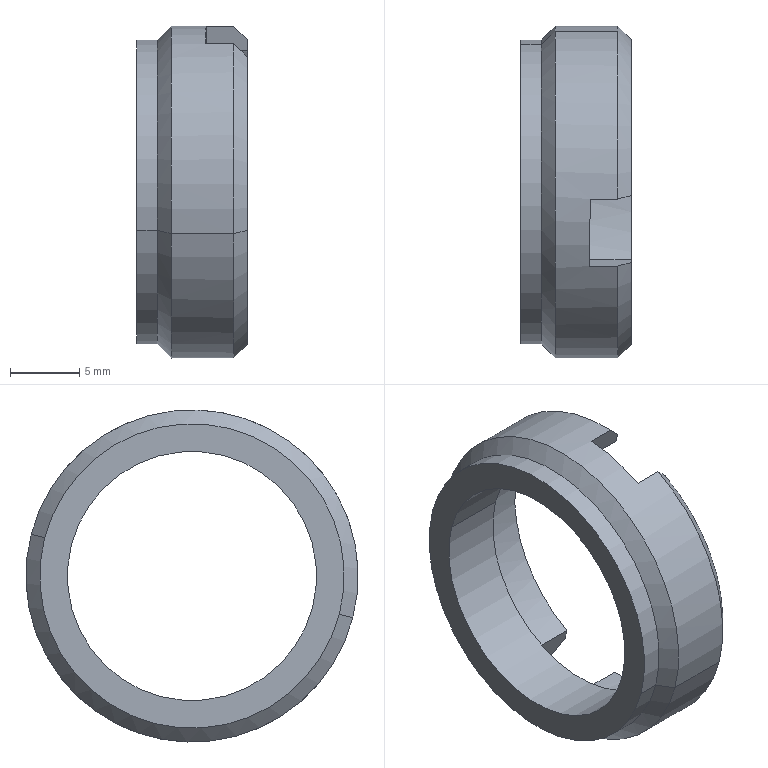Part | SolidWorks | features BaseBody 1 | 1 solid | 23 faces | box 8 x 24 x 24 mm | volume 1089 mm3 | plane 10 | cylinder 8 | cone 5 | commonest cylinder face diameters 18 x2 20.5 x2 22 x2 24 x2
STEP:
#1=CARTESIAN_POINT('',(259.5,87.353,-18.764));
#2=VERTEX_POINT('',#1);
#3=CARTESIAN_POINT('',(259.5,108.647,-13.236));
#4=VERTEX_POINT('',#3);
#5=CARTESIAN_POINT('',(259.5,98.,-16.));
#6=DIRECTION('',(-1.,0.,0.));
#7=DIRECTION('',(0.,-0.9679,-0.2513));
#8=AXIS2_PLACEMENT_3D('',#5,#6,#7);
#9=CIRCLE('',#8,11.);
#10=EDGE_CURVE('',#2,#4,#9,.T.);
#11=ORIENTED_EDGE('',*,*,#10,.F.);
#12=CARTESIAN_POINT('',(260.5,86.385,-19.015));
#13=VERTEX_POINT('',#12);
#14=CARTESIAN_POINT('',(259.5,87.353,-18.764));
#15=DIRECTION('',(0.7071,-0.6844,-0.1777));
#16=VECTOR('',#15,1000.);
#17=LINE('',#14,#16);
#18=EDGE_CURVE('',#2,#13,#17,.T.);
#19=ORIENTED_EDGE('',*,*,#18,.T.);
#20=CARTESIAN_POINT('',(260.5,109.615,-12.985));
#21=VERTEX_POINT('',#20);
#22=CARTESIAN_POINT('',(260.5,98.,-16.));
#23=DIRECTION('',(1.,0.,0.));
#24=DIRECTION('',(0.,-0.9679,-0.2513));
#25=AXIS2_PLACEMENT_3D('',#22,#23,#24);
#26=CIRCLE('',#25,12.);
#27=EDGE_CURVE('',#21,#13,#26,.T.);
#28=ORIENTED_EDGE('',*,*,#27,.F.);
#29=CARTESIAN_POINT('',(259.5,108.647,-13.236));
#30=DIRECTION('',(0.7071,0.6844,0.1777));
#31=VECTOR('',#30,1000.);
#32=LINE('',#29,#31);
#33=EDGE_CURVE('',#4,#21,#32,.T.);
#34=ORIENTED_EDGE('',*,*,#33,.F.);
#35=EDGE_LOOP('',(#11,#19,#28,#34));
#36=FACE_OUTER_BOUND('',#35,.T.);
#37=CARTESIAN_POINT('',(259.5,98.,-16.));
#38=DIRECTION('',(1.,0.,0.));
#39=DIRECTION('',(0.,0.9679,0.2513));
#40=AXIS2_PLACEMENT_3D('',#37,#38,#39);
#41=CONICAL_SURFACE('',#40,11.,0.7854);
#42=ADVANCED_FACE('',(#36),#41,.T.);
#43=CARTESIAN_POINT('',(266.,87.353,-18.764));
#44=VERTEX_POINT('',#43);
#45=CARTESIAN_POINT('',(266.,98.272,-26.997));
#46=VERTEX_POINT('',#45);
#47=CARTESIAN_POINT('',(266.,98.,-16.));
#48=DIRECTION('',(1.,0.,0.));
#49=DIRECTION('',(0.,-0.9679,-0.2513));
#50=AXIS2_PLACEMENT_3D('',#47,#48,#49);
#51=CIRCLE('',#50,11.);
#52=EDGE_CURVE('',#44,#46,#51,.T.);
#53=ORIENTED_EDGE('',*,*,#52,.F.);
#54=CARTESIAN_POINT('',(265.,86.385,-19.015));
#55=VERTEX_POINT('',#54);
#56=CARTESIAN_POINT('',(265.,86.385,-19.015));
#57=DIRECTION('',(-0.7071,-0.6844,-0.1777));
#58=VECTOR('',#57,1000.);
#59=LINE('',#56,#58);
#60=EDGE_CURVE('',#44,#55,#59,.T.);
#61=ORIENTED_EDGE('',*,*,#60,.T.);
#62=CARTESIAN_POINT('',(265.,98.529,-27.988));
#63=VERTEX_POINT('',#62);
#64=CARTESIAN_POINT('',(265.,98.,-16.));
#65=DIRECTION('',(-1.,0.,0.));
#66=DIRECTION('',(0.,-0.9679,-0.2513));
#67=AXIS2_PLACEMENT_3D('',#64,#65,#66);
#68=CIRCLE('',#67,12.);
#69=EDGE_CURVE('',#63,#55,#68,.T.);
#70=ORIENTED_EDGE('',*,*,#69,.F.);
#71=CARTESIAN_POINT('',(266.,98.272,-26.997));
#72=CARTESIAN_POINT('',(265.667,98.358,-27.328));
#73=CARTESIAN_POINT('',(265.334,98.443,-27.658));
#74=CARTESIAN_POINT('',(265.,98.529,-27.988));
#75=B_SPLINE_CURVE_WITH_KNOTS('',3,(#71,#72,#73,#74),.UNSPECIFIED.,.F.,.F.,(4,4),(0.04958,0.051),.UNSPECIFIED.);
#76=EDGE_CURVE('',#46,#63,#75,.T.);
#77=ORIENTED_EDGE('',*,*,#76,.F.);
#78=EDGE_LOOP('',(#53,#61,#70,#77));
#79=FACE_OUTER_BOUND('',#78,.T.);
#80=CARTESIAN_POINT('',(265.,98.,-16.));
#81=DIRECTION('',(-1.,0.,0.));
#82=DIRECTION('',(0.,-0.9679,-0.2513));
#83=AXIS2_PLACEMENT_3D('',#80,#81,#82);
#84=CONICAL_SURFACE('',#83,12.,0.7854);
#85=ADVANCED_FACE('',(#79),#84,.T.);
#86=CARTESIAN_POINT('',(258.,89.289,-18.261));
#87=VERTEX_POINT('',#86);
#88=CARTESIAN_POINT('',(258.,106.711,-13.739));
#89=VERTEX_POINT('',#88);
#90=CARTESIAN_POINT('',(258.,98.,-16.));
#91=DIRECTION('',(1.,0.,0.));
#92=DIRECTION('',(0.,0.9679,0.2513));
#93=AXIS2_PLACEMENT_3D('',#90,#91,#92);
#94=CIRCLE('',#93,9.);
#95=EDGE_CURVE('',#87,#89,#94,.T.);
#96=ORIENTED_EDGE('',*,*,#95,.F.);
#97=CARTESIAN_POINT('',(262.5,89.289,-18.261));
#98=VERTEX_POINT('',#97);
#99=CARTESIAN_POINT('',(258.,89.289,-18.261));
#100=DIRECTION('',(1.,0.,0.));
#101=VECTOR('',#100,1000.);
#102=LINE('',#99,#101);
#103=EDGE_CURVE('',#87,#98,#102,.T.);
#104=ORIENTED_EDGE('',*,*,#103,.T.);
#105=CARTESIAN_POINT('',(262.5,106.711,-13.739));
#106=VERTEX_POINT('',#105);
#107=CARTESIAN_POINT('',(262.5,98.,-16.));
#108=DIRECTION('',(1.,0.,0.));
#109=DIRECTION('',(0.,0.9679,0.2513));
#110=AXIS2_PLACEMENT_3D('',#107,#108,#109);
#111=CIRCLE('',#110,9.);
#112=EDGE_CURVE('',#98,#106,#111,.T.);
#113=ORIENTED_EDGE('',*,*,#112,.T.);
#114=CARTESIAN_POINT('',(258.,106.711,-13.739));
#115=DIRECTION('',(1.,0.,0.));
#116=VECTOR('',#115,1000.);
#117=LINE('',#114,#116);
#118=EDGE_CURVE('',#89,#106,#117,.T.);
#119=ORIENTED_EDGE('',*,*,#118,.F.);
#120=EDGE_LOOP('',(#96,#104,#113,#119));
#121=FACE_OUTER_BOUND('',#120,.T.);
#122=CARTESIAN_POINT('',(258.,98.,-16.));
#123=DIRECTION('',(1.,0.,0.));
#124=DIRECTION('',(0.,0.9679,0.2513));
#125=AXIS2_PLACEMENT_3D('',#122,#123,#124);
#126=CYLINDRICAL_SURFACE('',#125,9.);
#127=ADVANCED_FACE('',(#121),#126,.F.);
#128=CARTESIAN_POINT('',(262.5,88.079,-18.575));
#129=VERTEX_POINT('',#128);
#130=CARTESIAN_POINT('',(262.5,107.921,-13.425));
#131=VERTEX_POINT('',#130);
#132=CARTESIAN_POINT('',(262.5,98.,-16.));
#133=DIRECTION('',(1.,0.,0.));
#134=DIRECTION('',(0.,0.9679,0.2513));
#135=AXIS2_PLACEMENT_3D('',#132,#133,#134);
#136=CIRCLE('',#135,10.25);
#137=EDGE_CURVE('',#129,#131,#136,.T.);
#138=ORIENTED_EDGE('',*,*,#137,.F.);
#139=CARTESIAN_POINT('',(266.,88.079,-18.575));
#140=VERTEX_POINT('',#139);
#141=CARTESIAN_POINT('',(262.5,88.079,-18.575));
#142=DIRECTION('',(1.,0.,0.));
#143=VECTOR('',#142,1000.);
#144=LINE('',#141,#143);
#145=EDGE_CURVE('',#129,#140,#144,.T.);
#146=ORIENTED_EDGE('',*,*,#145,.T.);
#147=CARTESIAN_POINT('',(266.,98.078,-26.25));
#148=VERTEX_POINT('',#147);
#149=CARTESIAN_POINT('',(266.,98.,-16.));
#150=DIRECTION('',(1.,0.,0.));
#151=DIRECTION('',(0.,0.9679,0.2513));
#152=AXIS2_PLACEMENT_3D('',#149,#150,#151);
#153=CIRCLE('',#152,10.25);
#154=EDGE_CURVE('',#140,#148,#153,.T.);
#155=ORIENTED_EDGE('',*,*,#154,.T.);
#156=CARTESIAN_POINT('',(262.973,98.078,-26.25));
#157=VERTEX_POINT('',#156);
#158=CARTESIAN_POINT('',(262.5,98.078,-26.25));
#159=DIRECTION('',(-1.,0.,0.));
#160=VECTOR('',#159,1000.);
#161=LINE('',#158,#160);
#162=EDGE_CURVE('',#148,#157,#161,.T.);
#163=ORIENTED_EDGE('',*,*,#162,.T.);
#164=CARTESIAN_POINT('',(263.027,102.917,-24.993));
#165=VERTEX_POINT('',#164);
#166=CARTESIAN_POINT('',(262.973,98.078,-26.25));
#167=CARTESIAN_POINT('',(262.991,99.779,-26.237));
#168=CARTESIAN_POINT('',(263.009,101.425,-25.809));
#169=CARTESIAN_POINT('',(263.027,102.917,-24.993));
#170=(BOUNDED_CURVE()B_SPLINE_CURVE(3,(#166,#167,#168,#169),.UNSPECIFIED.,.F.,.F.)B_SPLINE_CURVE_WITH_KNOTS((4,4),(4.466,4.959),.UNSPECIFIED.)CURVE()GEOMETRIC_REPRESENTATION_ITEM()RATIONAL_B_SPLINE_CURVE((1.,0.9799,0.9799,1.))REPRESENTATION_ITEM(''));
#171=EDGE_CURVE('',#157,#165,#170,.T.);
#172=ORIENTED_EDGE('',*,*,#171,.T.);
#173=CARTESIAN_POINT('',(266.,102.917,-24.993));
#174=VERTEX_POINT('',#173);
#175=CARTESIAN_POINT('',(262.5,102.917,-24.993));
#176=DIRECTION('',(1.,0.,0.));
#177=VECTOR('',#176,1000.);
#178=LINE('',#175,#177);
#179=EDGE_CURVE('',#165,#174,#178,.T.);
#180=ORIENTED_EDGE('',*,*,#179,.T.);
#181=CARTESIAN_POINT('',(266.,107.921,-13.425));
#182=VERTEX_POINT('',#181);
#183=CARTESIAN_POINT('',(266.,98.,-16.));
#184=DIRECTION('',(1.,0.,0.));
#185=DIRECTION('',(0.,0.9679,0.2513));
#186=AXIS2_PLACEMENT_3D('',#183,#184,#185);
#187=CIRCLE('',#186,10.25);
#188=EDGE_CURVE('',#174,#182,#187,.T.);
#189=ORIENTED_EDGE('',*,*,#188,.T.);
#190=CARTESIAN_POINT('',(262.5,107.921,-13.425));
#191=DIRECTION('',(1.,0.,0.));
#192=VECTOR('',#191,1000.);
#193=LINE('',#190,#192);
#194=EDGE_CURVE('',#131,#182,#193,.T.);
#195=ORIENTED_EDGE('',*,*,#194,.F.);
#196=EDGE_LOOP('',(#138,#146,#155,#163,#172,#180,#189,#195));
#197=FACE_OUTER_BOUND('',#196,.T.);
#198=CARTESIAN_POINT('',(262.5,98.,-16.));
#199=DIRECTION('',(1.,0.,0.));
#200=DIRECTION('',(0.,0.9679,0.2513));
#201=AXIS2_PLACEMENT_3D('',#198,#199,#200);
#202=CYLINDRICAL_SURFACE('',#201,10.25);
#203=ADVANCED_FACE('',(#197),#202,.F.);
#204=CARTESIAN_POINT('',(258.,87.353,-18.764));
#205=VERTEX_POINT('',#204);
#206=CARTESIAN_POINT('',(258.,108.647,-13.236));
#207=VERTEX_POINT('',#206);
#208=CARTESIAN_POINT('',(258.,98.,-16.));
#209=DIRECTION('',(-1.,0.,0.));
#210=DIRECTION('',(0.,-0.9679,-0.2513));
#211=AXIS2_PLACEMENT_3D('',#208,#209,#210);
#212=CIRCLE('',#211,11.);
#213=EDGE_CURVE('',#205,#207,#212,.T.);
#214=ORIENTED_EDGE('',*,*,#213,.F.);
#215=CARTESIAN_POINT('',(258.,87.353,-18.764));
#216=DIRECTION('',(1.,0.,0.));
#217=VECTOR('',#216,1000.);
#218=LINE('',#215,#217);
#219=EDGE_CURVE('',#205,#2,#218,.T.);
#220=ORIENTED_EDGE('',*,*,#219,.T.);
#221=ORIENTED_EDGE('',*,*,#10,.T.);
#222=CARTESIAN_POINT('',(258.,108.647,-13.236));
#223=DIRECTION('',(1.,0.,0.));
#224=VECTOR('',#223,1000.);
#225=LINE('',#222,#224);
#226=EDGE_CURVE('',#207,#4,#225,.T.);
#227=ORIENTED_EDGE('',*,*,#226,.F.);
#228=EDGE_LOOP('',(#214,#220,#221,#227));
#229=FACE_OUTER_BOUND('',#228,.T.);
#230=CARTESIAN_POINT('',(258.,98.,-16.));
#231=DIRECTION('',(1.,0.,0.));
#232=DIRECTION('',(0.,0.9679,0.2513));
#233=AXIS2_PLACEMENT_3D('',#230,#231,#232);
#234=CYLINDRICAL_SURFACE('',#233,11.);
#235=ADVANCED_FACE('',(#229),#234,.T.);
#236=ORIENTED_EDGE('',*,*,#27,.T.);
#237=CARTESIAN_POINT('',(259.5,86.385,-19.015));
#238=DIRECTION('',(1.,0.,0.));
#239=VECTOR('',#238,1000.);
#240=LINE('',#237,#239);
#241=EDGE_CURVE('',#13,#55,#240,.T.);
#242=ORIENTED_EDGE('',*,*,#241,.T.);
#243=CARTESIAN_POINT('',(265.,92.631,-5.268));
#244=VERTEX_POINT('',#243);
#245=CARTESIAN_POINT('',(265.,98.,-16.));
#246=DIRECTION('',(-1.,0.,0.));
#247=DIRECTION('',(0.,-0.9679,-0.2513));
#248=AXIS2_PLACEMENT_3D('',#245,#246,#247);
#249=CIRCLE('',#248,12.);
#250=EDGE_CURVE('',#55,#244,#249,.T.);
#251=ORIENTED_EDGE('',*,*,#250,.T.);
#252=CARTESIAN_POINT('',(262.973,92.631,-5.268));
#253=VERTEX_POINT('',#252);
#254=CARTESIAN_POINT('',(259.5,92.631,-5.268));
#255=DIRECTION('',(-1.,0.,0.));
#256=VECTOR('',#255,1000.);
#257=LINE('',#254,#256);
#258=EDGE_CURVE('',#244,#253,#257,.T.);
#259=ORIENTED_EDGE('',*,*,#258,.T.);
#260=CARTESIAN_POINT('',(263.027,97.471,-4.012));
#261=VERTEX_POINT('',#260);
#262=CARTESIAN_POINT('',(262.973,92.631,-5.268));
#263=CARTESIAN_POINT('',(262.991,94.144,-4.511));
#264=CARTESIAN_POINT('',(263.009,95.781,-4.086));
#265=CARTESIAN_POINT('',(263.027,97.471,-4.012));
#266=(BOUNDED_CURVE()B_SPLINE_CURVE(3,(#262,#263,#264,#265),.UNSPECIFIED.,.F.,.T.)B_SPLINE_CURVE_WITH_KNOTS((4,4),(4.503,4.922),.UNSPECIFIED.)CURVE()GEOMETRIC_REPRESENTATION_ITEM()RATIONAL_B_SPLINE_CURVE((1.,0.9854,0.9854,1.))REPRESENTATION_ITEM(''));
#267=EDGE_CURVE('',#253,#261,#266,.T.);
#268=ORIENTED_EDGE('',*,*,#267,.T.);
#269=CARTESIAN_POINT('',(265.,97.471,-4.012));
#270=VERTEX_POINT('',#269);
#271=CARTESIAN_POINT('',(259.5,97.471,-4.012));
#272=DIRECTION('',(1.,0.,0.));
#273=VECTOR('',#272,1000.);
#274=LINE('',#271,#273);
#275=EDGE_CURVE('',#261,#270,#274,.T.);
#276=ORIENTED_EDGE('',*,*,#275,.T.);
#277=CARTESIAN_POINT('',(265.,109.615,-12.985));
#278=VERTEX_POINT('',#277);
#279=CARTESIAN_POINT('',(265.,98.,-16.));
#280=DIRECTION('',(-1.,0.,0.));
#281=DIRECTION('',(0.,-0.9679,-0.2513));
#282=AXIS2_PLACEMENT_3D('',#279,#280,#281);
#283=CIRCLE('',#282,12.);
#284=EDGE_CURVE('',#270,#278,#283,.T.);
#285=ORIENTED_EDGE('',*,*,#284,.T.);
#286=CARTESIAN_POINT('',(259.5,109.615,-12.985));
#287=DIRECTION('',(1.,0.,0.));
#288=VECTOR('',#287,1000.);
#289=LINE('',#286,#288);
#290=EDGE_CURVE('',#21,#278,#289,.T.);
#291=ORIENTED_EDGE('',*,*,#290,.F.);
#292=EDGE_LOOP('',(#236,#242,#251,#259,#268,#276,#285,#291));
#293=FACE_OUTER_BOUND('',#292,.T.);
#294=CARTESIAN_POINT('',(259.5,98.,-16.));
#295=DIRECTION('',(1.,0.,0.));
#296=DIRECTION('',(0.,0.9679,0.2513));
#297=AXIS2_PLACEMENT_3D('',#294,#295,#296);
#298=CYLINDRICAL_SURFACE('',#297,12.);
#299=ADVANCED_FACE('',(#293),#298,.T.);
#300=CARTESIAN_POINT('',(266.,103.111,-25.74));
#301=VERTEX_POINT('',#300);
#302=CARTESIAN_POINT('',(266.,97.728,-5.003));
#303=VERTEX_POINT('',#302);
#304=CARTESIAN_POINT('',(266.,98.,-16.));
#305=DIRECTION('',(1.,0.,0.));
#306=DIRECTION('',(0.,-0.9679,-0.2513));
#307=AXIS2_PLACEMENT_3D('',#304,#305,#306);
#308=CIRCLE('',#307,11.);
#309=EDGE_CURVE('',#301,#303,#308,.T.);
#310=ORIENTED_EDGE('',*,*,#309,.T.);
#311=CARTESIAN_POINT('',(266.,97.922,-5.75));
#312=VERTEX_POINT('',#311);
#313=CARTESIAN_POINT('',(266.,103.435,-26.987));
#314=DIRECTION('',(0.,-0.2513,0.9679));
#315=VECTOR('',#314,1000.);
#316=LINE('',#313,#315);
#317=EDGE_CURVE('',#312,#303,#316,.T.);
#318=ORIENTED_EDGE('',*,*,#317,.F.);
#319=CARTESIAN_POINT('',(266.,98.,-16.));
#320=DIRECTION('',(1.,0.,0.));
#321=DIRECTION('',(0.,0.9679,0.2513));
#322=AXIS2_PLACEMENT_3D('',#319,#320,#321);
#323=CIRCLE('',#322,10.25);
#324=EDGE_CURVE('',#182,#312,#323,.T.);
#325=ORIENTED_EDGE('',*,*,#324,.F.);
#326=ORIENTED_EDGE('',*,*,#188,.F.);
#327=CARTESIAN_POINT('',(266.,103.435,-26.987));
#328=DIRECTION('',(0.,-0.2513,0.9679));
#329=VECTOR('',#328,1000.);
#330=LINE('',#327,#329);
#331=EDGE_CURVE('',#301,#174,#330,.T.);
#332=ORIENTED_EDGE('',*,*,#331,.F.);
#333=EDGE_LOOP('',(#310,#318,#325,#326,#332));
#334=FACE_OUTER_BOUND('',#333,.T.);
#335=CARTESIAN_POINT('',(266.,98.,-16.));
#336=DIRECTION('',(-1.,0.,0.));
#337=DIRECTION('',(0.,-0.9679,-0.2513));
#338=AXIS2_PLACEMENT_3D('',#335,#336,#337);
#339=PLANE('',#338);
#340=ADVANCED_FACE('',(#334),#339,.F.);
#341=CARTESIAN_POINT('',(265.,103.369,-26.732));
#342=VERTEX_POINT('',#341);
#343=CARTESIAN_POINT('',(265.,103.369,-26.732));
#344=CARTESIAN_POINT('',(265.334,103.283,-26.402));
#345=CARTESIAN_POINT('',(265.667,103.197,-26.071));
#346=CARTESIAN_POINT('',(266.,103.111,-25.74));
#347=B_SPLINE_CURVE_WITH_KNOTS('',3,(#343,#344,#345,#346),.UNSPECIFIED.,.F.,.F.,(4,4),(0.02048,0.02192),.UNSPECIFIED.);
#348=EDGE_CURVE('',#342,#301,#347,.T.);
#349=ORIENTED_EDGE('',*,*,#348,.F.);
#350=CARTESIAN_POINT('',(265.,98.,-16.));
#351=DIRECTION('',(-1.,0.,0.));
#352=DIRECTION('',(0.,-0.9679,-0.2513));
#353=AXIS2_PLACEMENT_3D('',#350,#351,#352);
#354=CIRCLE('',#353,12.);
#355=EDGE_CURVE('',#278,#342,#354,.T.);
#356=ORIENTED_EDGE('',*,*,#355,.F.);
#357=ORIENTED_EDGE('',*,*,#284,.F.);
#358=CARTESIAN_POINT('',(266.,97.728,-5.003));
#359=CARTESIAN_POINT('',(265.667,97.642,-4.672));
#360=CARTESIAN_POINT('',(265.334,97.557,-4.342));
#361=CARTESIAN_POINT('',(265.,97.471,-4.012));
#362=B_SPLINE_CURVE_WITH_KNOTS('',3,(#358,#359,#360,#361),.UNSPECIFIED.,.F.,.F.,(4,4),(0.04958,0.051),.UNSPECIFIED.);
#363=EDGE_CURVE('',#303,#270,#362,.T.);
#364=ORIENTED_EDGE('',*,*,#363,.F.);
#365=ORIENTED_EDGE('',*,*,#309,.F.);
#366=EDGE_LOOP('',(#349,#356,#357,#364,#365));
#367=FACE_OUTER_BOUND('',#366,.T.);
#368=CARTESIAN_POINT('',(265.,98.,-16.));
#369=DIRECTION('',(-1.,0.,0.));
#370=DIRECTION('',(0.,-0.9679,-0.2513));
#371=AXIS2_PLACEMENT_3D('',#368,#369,#370);
#372=CONICAL_SURFACE('',#371,12.,0.7854);
#373=ADVANCED_FACE('',(#367),#372,.T.);
#374=ORIENTED_EDGE('',*,*,#241,.F.);
#375=CARTESIAN_POINT('',(260.5,98.,-16.));
#376=DIRECTION('',(1.,0.,0.));
#377=DIRECTION('',(0.,-0.9679,-0.2513));
#378=AXIS2_PLACEMENT_3D('',#375,#376,#377);
#379=CIRCLE('',#378,12.);
#380=EDGE_CURVE('',#13,#21,#379,.T.);
#381=ORIENTED_EDGE('',*,*,#380,.T.);
#382=ORIENTED_EDGE('',*,*,#290,.T.);
#383=ORIENTED_EDGE('',*,*,#355,.T.);
#384=CARTESIAN_POINT('',(263.027,103.369,-26.732));
#385=VERTEX_POINT('',#384);
#386=CARTESIAN_POINT('',(259.5,103.369,-26.732));
#387=DIRECTION('',(-1.,0.,0.));
#388=VECTOR('',#387,1000.);
#389=LINE('',#386,#388);
#390=EDGE_CURVE('',#342,#385,#389,.T.);
#391=ORIENTED_EDGE('',*,*,#390,.T.);
#392=CARTESIAN_POINT('',(262.973,98.529,-27.988));
#393=VERTEX_POINT('',#392);
#394=CARTESIAN_POINT('',(263.027,103.369,-26.732));
#395=CARTESIAN_POINT('',(263.009,101.856,-27.489));
#396=CARTESIAN_POINT('',(262.991,100.219,-27.914));
#397=CARTESIAN_POINT('',(262.973,98.529,-27.988));
#398=(BOUNDED_CURVE()B_SPLINE_CURVE(3,(#394,#395,#396,#397),.UNSPECIFIED.,.F.,.F.)B_SPLINE_CURVE_WITH_KNOTS((4,4),(1.361,1.781),.UNSPECIFIED.)CURVE()GEOMETRIC_REPRESENTATION_ITEM()RATIONAL_B_SPLINE_CURVE((1.,0.9854,0.9854,1.))REPRESENTATION_ITEM(''));
#399=EDGE_CURVE('',#385,#393,#398,.T.);
#400=ORIENTED_EDGE('',*,*,#399,.T.);
#401=CARTESIAN_POINT('',(259.5,98.529,-27.988));
#402=DIRECTION('',(1.,0.,0.));
#403=VECTOR('',#402,1000.);
#404=LINE('',#401,#403);
#405=EDGE_CURVE('',#393,#63,#404,.T.);
#406=ORIENTED_EDGE('',*,*,#405,.T.);
#407=ORIENTED_EDGE('',*,*,#69,.T.);
#408=EDGE_LOOP('',(#374,#381,#382,#383,#391,#400,#406,#407));
#409=FACE_OUTER_BOUND('',#408,.T.);
#410=CARTESIAN_POINT('',(259.5,98.,-16.));
#411=DIRECTION('',(1.,0.,0.));
#412=DIRECTION('',(0.,0.9679,0.2513));
#413=AXIS2_PLACEMENT_3D('',#410,#411,#412);
#414=CYLINDRICAL_SURFACE('',#413,12.);
#415=ADVANCED_FACE('',(#409),#414,.T.);
#416=CARTESIAN_POINT('',(266.,92.889,-6.26));
#417=VERTEX_POINT('',#416);
#418=CARTESIAN_POINT('',(266.,98.,-16.));
#419=DIRECTION('',(1.,0.,0.));
#420=DIRECTION('',(0.,-0.9679,-0.2513));
#421=AXIS2_PLACEMENT_3D('',#418,#419,#420);
#422=CIRCLE('',#421,11.);
#423=EDGE_CURVE('',#417,#44,#422,.T.);
#424=ORIENTED_EDGE('',*,*,#423,.T.);
#425=ORIENTED_EDGE('',*,*,#52,.T.);
#426=CARTESIAN_POINT('',(266.,98.595,-28.243));
#427=DIRECTION('',(0.,-0.2513,0.9679));
#428=VECTOR('',#427,1000.);
#429=LINE('',#426,#428);
#430=EDGE_CURVE('',#46,#148,#429,.T.);
#431=ORIENTED_EDGE('',*,*,#430,.T.);
#432=ORIENTED_EDGE('',*,*,#154,.F.);
#433=CARTESIAN_POINT('',(266.,93.083,-7.007));
#434=VERTEX_POINT('',#433);
#435=CARTESIAN_POINT('',(266.,98.,-16.));
#436=DIRECTION('',(1.,0.,0.));
#437=DIRECTION('',(0.,0.9679,0.2513));
#438=AXIS2_PLACEMENT_3D('',#435,#436,#437);
#439=CIRCLE('',#438,10.25);
#440=EDGE_CURVE('',#434,#140,#439,.T.);
#441=ORIENTED_EDGE('',*,*,#440,.F.);
#442=CARTESIAN_POINT('',(266.,98.595,-28.243));
#443=DIRECTION('',(0.,-0.2513,0.9679));
#444=VECTOR('',#443,1000.);
#445=LINE('',#442,#444);
#446=EDGE_CURVE('',#434,#417,#445,.T.);
#447=ORIENTED_EDGE('',*,*,#446,.T.);
#448=EDGE_LOOP('',(#424,#425,#431,#432,#441,#447));
#449=FACE_OUTER_BOUND('',#448,.T.);
#450=CARTESIAN_POINT('',(266.,98.,-16.));
#451=DIRECTION('',(-1.,0.,0.));
#452=DIRECTION('',(0.,-0.9679,-0.2513));
#453=AXIS2_PLACEMENT_3D('',#450,#451,#452);
#454=PLANE('',#453);
#455=ADVANCED_FACE('',(#449),#454,.F.);
#456=ORIENTED_EDGE('',*,*,#219,.F.);
#457=CARTESIAN_POINT('',(258.,98.,-16.));
#458=DIRECTION('',(-1.,0.,0.));
#459=DIRECTION('',(0.,-0.9679,-0.2513));
#460=AXIS2_PLACEMENT_3D('',#457,#458,#459);
#461=CIRCLE('',#460,11.);
#462=EDGE_CURVE('',#207,#205,#461,.T.);
#463=ORIENTED_EDGE('',*,*,#462,.F.);
#464=ORIENTED_EDGE('',*,*,#226,.T.);
#465=CARTESIAN_POINT('',(259.5,98.,-16.));
#466=DIRECTION('',(-1.,0.,0.));
#467=DIRECTION('',(0.,-0.9679,-0.2513));
#468=AXIS2_PLACEMENT_3D('',#465,#466,#467);
#469=CIRCLE('',#468,11.);
#470=EDGE_CURVE('',#4,#2,#469,.T.);
#471=ORIENTED_EDGE('',*,*,#470,.T.);
#472=EDGE_LOOP('',(#456,#463,#464,#471));
#473=FACE_OUTER_BOUND('',#472,.T.);
#474=CARTESIAN_POINT('',(258.,98.,-16.));
#475=DIRECTION('',(1.,0.,0.));
#476=DIRECTION('',(0.,0.9679,0.2513));
#477=AXIS2_PLACEMENT_3D('',#474,#475,#476);
#478=CYLINDRICAL_SURFACE('',#477,11.);
#479=ADVANCED_FACE('',(#473),#478,.T.);
#480=CARTESIAN_POINT('',(258.,98.,-16.));
#481=DIRECTION('',(1.,0.,0.));
#482=DIRECTION('',(0.,0.9679,0.2513));
#483=AXIS2_PLACEMENT_3D('',#480,#481,#482);
#484=CIRCLE('',#483,9.);
#485=EDGE_CURVE('',#89,#87,#484,.T.);
#486=ORIENTED_EDGE('',*,*,#485,.T.);
#487=ORIENTED_EDGE('',*,*,#95,.T.);
#488=EDGE_LOOP('',(#486,#487));
#489=FACE_BOUND('',#488,.T.);
#490=ORIENTED_EDGE('',*,*,#462,.T.);
#491=ORIENTED_EDGE('',*,*,#213,.T.);
#492=EDGE_LOOP('',(#490,#491));
#493=FACE_OUTER_BOUND('',#492,.T.);
#494=CARTESIAN_POINT('',(258.,98.,-16.));
#495=DIRECTION('',(-1.,0.,0.));
#496=DIRECTION('',(0.,-0.9679,-0.2513));
#497=AXIS2_PLACEMENT_3D('',#494,#495,#496);
#498=PLANE('',#497);
#499=ADVANCED_FACE('',(#489,#493),#498,.T.);
#500=ORIENTED_EDGE('',*,*,#145,.F.);
#501=CARTESIAN_POINT('',(262.5,98.,-16.));
#502=DIRECTION('',(1.,0.,0.));
#503=DIRECTION('',(0.,0.9679,0.2513));
#504=AXIS2_PLACEMENT_3D('',#501,#502,#503);
#505=CIRCLE('',#504,10.25);
#506=EDGE_CURVE('',#131,#129,#505,.T.);
#507=ORIENTED_EDGE('',*,*,#506,.F.);
#508=ORIENTED_EDGE('',*,*,#194,.T.);
#509=ORIENTED_EDGE('',*,*,#324,.T.);
#510=CARTESIAN_POINT('',(263.027,97.922,-5.75));
#511=VERTEX_POINT('',#510);
#512=CARTESIAN_POINT('',(262.5,97.922,-5.75));
#513=DIRECTION('',(-1.,0.,0.));
#514=VECTOR('',#513,1000.);
#515=LINE('',#512,#514);
#516=EDGE_CURVE('',#312,#511,#515,.T.);
#517=ORIENTED_EDGE('',*,*,#516,.T.);
#518=CARTESIAN_POINT('',(262.973,93.083,-7.007));
#519=VERTEX_POINT('',#518);
#520=CARTESIAN_POINT('',(263.027,97.922,-5.75));
#521=CARTESIAN_POINT('',(263.009,96.221,-5.763));
#522=CARTESIAN_POINT('',(262.991,94.575,-6.191));
#523=CARTESIAN_POINT('',(262.973,93.083,-7.007));
#524=(BOUNDED_CURVE()B_SPLINE_CURVE(3,(#520,#521,#522,#523),.UNSPECIFIED.,.F.,.F.)B_SPLINE_CURVE_WITH_KNOTS((4,4),(1.324,1.817),.UNSPECIFIED.)CURVE()GEOMETRIC_REPRESENTATION_ITEM()RATIONAL_B_SPLINE_CURVE((1.,0.9799,0.9799,1.))REPRESENTATION_ITEM(''));
#525=EDGE_CURVE('',#511,#519,#524,.T.);
#526=ORIENTED_EDGE('',*,*,#525,.T.);
#527=CARTESIAN_POINT('',(262.5,93.083,-7.007));
#528=DIRECTION('',(1.,0.,0.));
#529=VECTOR('',#528,1000.);
#530=LINE('',#527,#529);
#531=EDGE_CURVE('',#519,#434,#530,.T.);
#532=ORIENTED_EDGE('',*,*,#531,.T.);
#533=ORIENTED_EDGE('',*,*,#440,.T.);
#534=EDGE_LOOP('',(#500,#507,#508,#509,#517,#526,#532,#533));
#535=FACE_OUTER_BOUND('',#534,.T.);
#536=CARTESIAN_POINT('',(262.5,98.,-16.));
#537=DIRECTION('',(1.,0.,0.));
#538=DIRECTION('',(0.,0.9679,0.2513));
#539=AXIS2_PLACEMENT_3D('',#536,#537,#538);
#540=CYLINDRICAL_SURFACE('',#539,10.25);
#541=ADVANCED_FACE('',(#535),#540,.F.);
#542=CARTESIAN_POINT('',(262.5,98.,-16.));
#543=DIRECTION('',(1.,0.,0.));
#544=DIRECTION('',(0.,0.9679,0.2513));
#545=AXIS2_PLACEMENT_3D('',#542,#543,#544);
#546=CIRCLE('',#545,9.);
#547=EDGE_CURVE('',#106,#98,#546,.T.);
#548=ORIENTED_EDGE('',*,*,#547,.F.);
#549=ORIENTED_EDGE('',*,*,#112,.F.);
#550=EDGE_LOOP('',(#548,#549));
#551=FACE_BOUND('',#550,.T.);
#552=ORIENTED_EDGE('',*,*,#506,.T.);
#553=ORIENTED_EDGE('',*,*,#137,.T.);
#554=EDGE_LOOP('',(#552,#553));
#555=FACE_OUTER_BOUND('',#554,.T.);
#556=CARTESIAN_POINT('',(262.5,98.,-16.));
#557=DIRECTION('',(1.,0.,0.));
#558=DIRECTION('',(0.,0.9679,0.2513));
#559=AXIS2_PLACEMENT_3D('',#556,#557,#558);
#560=PLANE('',#559);
#561=ADVANCED_FACE('',(#551,#555),#560,.T.);
#562=ORIENTED_EDGE('',*,*,#103,.F.);
#563=ORIENTED_EDGE('',*,*,#485,.F.);
#564=ORIENTED_EDGE('',*,*,#118,.T.);
#565=ORIENTED_EDGE('',*,*,#547,.T.);
#566=EDGE_LOOP('',(#562,#563,#564,#565));
#567=FACE_OUTER_BOUND('',#566,.T.);
#568=CARTESIAN_POINT('',(258.,98.,-16.));
#569=DIRECTION('',(1.,0.,0.));
#570=DIRECTION('',(0.,0.9679,0.2513));
#571=AXIS2_PLACEMENT_3D('',#568,#569,#570);
#572=CYLINDRICAL_SURFACE('',#571,9.);
#573=ADVANCED_FACE('',(#567),#572,.F.);
#574=ORIENTED_EDGE('',*,*,#60,.F.);
#575=ORIENTED_EDGE('',*,*,#423,.F.);
#576=CARTESIAN_POINT('',(265.,92.631,-5.268));
#577=CARTESIAN_POINT('',(265.334,92.717,-5.598));
#578=CARTESIAN_POINT('',(265.667,92.803,-5.929));
#579=CARTESIAN_POINT('',(266.,92.889,-6.26));
#580=B_SPLINE_CURVE_WITH_KNOTS('',3,(#576,#577,#578,#579),.UNSPECIFIED.,.F.,.F.,(4,4),(0.02048,0.02192),.UNSPECIFIED.);
#581=EDGE_CURVE('',#244,#417,#580,.T.);
#582=ORIENTED_EDGE('',*,*,#581,.F.);
#583=ORIENTED_EDGE('',*,*,#250,.F.);
#584=EDGE_LOOP('',(#574,#575,#582,#583));
#585=FACE_OUTER_BOUND('',#584,.T.);
#586=CARTESIAN_POINT('',(265.,98.,-16.));
#587=DIRECTION('',(-1.,0.,0.));
#588=DIRECTION('',(0.,-0.9679,-0.2513));
#589=AXIS2_PLACEMENT_3D('',#586,#587,#588);
#590=CONICAL_SURFACE('',#589,12.,0.7854);
#591=ADVANCED_FACE('',(#585),#590,.T.);
#592=ORIENTED_EDGE('',*,*,#18,.F.);
#593=ORIENTED_EDGE('',*,*,#470,.F.);
#594=ORIENTED_EDGE('',*,*,#33,.T.);
#595=ORIENTED_EDGE('',*,*,#380,.F.);
#596=EDGE_LOOP('',(#592,#593,#594,#595));
#597=FACE_OUTER_BOUND('',#596,.T.);
#598=CARTESIAN_POINT('',(259.5,98.,-16.));
#599=DIRECTION('',(1.,0.,0.));
#600=DIRECTION('',(0.,0.9679,0.2513));
#601=AXIS2_PLACEMENT_3D('',#598,#599,#600);
#602=CONICAL_SURFACE('',#601,11.,0.7854);
#603=ADVANCED_FACE('',(#597),#602,.T.);
#604=ORIENTED_EDGE('',*,*,#430,.F.);
#605=ORIENTED_EDGE('',*,*,#76,.T.);
#606=ORIENTED_EDGE('',*,*,#405,.F.);
#607=CARTESIAN_POINT('',(262.973,98.595,-28.243));
#608=DIRECTION('',(0.,-0.2513,0.9679));
#609=VECTOR('',#608,1000.);
#610=LINE('',#607,#609);
#611=EDGE_CURVE('',#393,#157,#610,.T.);
#612=ORIENTED_EDGE('',*,*,#611,.T.);
#613=ORIENTED_EDGE('',*,*,#162,.F.);
#614=EDGE_LOOP('',(#604,#605,#606,#612,#613));
#615=FACE_OUTER_BOUND('',#614,.T.);
#616=CARTESIAN_POINT('',(266.,98.595,-28.243));
#617=DIRECTION('',(0.,-0.9679,-0.2513));
#618=DIRECTION('',(1.,0.,0.));
#619=AXIS2_PLACEMENT_3D('',#616,#617,#618);
#620=PLANE('',#619);
#621=ADVANCED_FACE('',(#615),#620,.F.);
#622=CARTESIAN_POINT('',(263.027,103.435,-26.987));
#623=DIRECTION('',(0.,-0.2513,0.9679));
#624=VECTOR('',#623,1000.);
#625=LINE('',#622,#624);
#626=EDGE_CURVE('',#385,#165,#625,.T.);
#627=ORIENTED_EDGE('',*,*,#626,.F.);
#628=ORIENTED_EDGE('',*,*,#390,.F.);
#629=ORIENTED_EDGE('',*,*,#348,.T.);
#630=ORIENTED_EDGE('',*,*,#331,.T.);
#631=ORIENTED_EDGE('',*,*,#179,.F.);
#632=EDGE_LOOP('',(#627,#628,#629,#630,#631));
#633=FACE_OUTER_BOUND('',#632,.T.);
#634=CARTESIAN_POINT('',(266.,103.435,-26.987));
#635=DIRECTION('',(0.,0.9679,0.2513));
#636=DIRECTION('',(-1.,0.,0.));
#637=AXIS2_PLACEMENT_3D('',#634,#635,#636);
#638=PLANE('',#637);
#639=ADVANCED_FACE('',(#633),#638,.F.);
#640=ORIENTED_EDGE('',*,*,#626,.T.);
#641=ORIENTED_EDGE('',*,*,#171,.F.);
#642=ORIENTED_EDGE('',*,*,#611,.F.);
#643=ORIENTED_EDGE('',*,*,#399,.F.);
#644=EDGE_LOOP('',(#640,#641,#642,#643));
#645=FACE_OUTER_BOUND('',#644,.T.);
#646=CARTESIAN_POINT('',(263.027,103.435,-26.987));
#647=DIRECTION('',(-0.9999,0.01042,0.002706));
#648=DIRECTION('',(-0.01077,-0.9679,-0.2512));
#649=AXIS2_PLACEMENT_3D('',#646,#647,#648);
#650=PLANE('',#649);
#651=ADVANCED_FACE('',(#645),#650,.F.);
#652=CARTESIAN_POINT('',(262.973,98.595,-28.243));
#653=DIRECTION('',(0.,-0.2513,0.9679));
#654=VECTOR('',#653,1000.);
#655=LINE('',#652,#654);
#656=EDGE_CURVE('',#519,#253,#655,.T.);
#657=ORIENTED_EDGE('',*,*,#656,.F.);
#658=ORIENTED_EDGE('',*,*,#525,.F.);
#659=CARTESIAN_POINT('',(263.027,103.435,-26.987));
#660=DIRECTION('',(0.,-0.2513,0.9679));
#661=VECTOR('',#660,1000.);
#662=LINE('',#659,#661);
#663=EDGE_CURVE('',#511,#261,#662,.T.);
#664=ORIENTED_EDGE('',*,*,#663,.T.);
#665=ORIENTED_EDGE('',*,*,#267,.F.);
#666=EDGE_LOOP('',(#657,#658,#664,#665));
#667=FACE_OUTER_BOUND('',#666,.T.);
#668=CARTESIAN_POINT('',(263.027,103.435,-26.987));
#669=DIRECTION('',(-0.9999,0.01042,0.002706));
#670=DIRECTION('',(-0.01077,-0.9679,-0.2512));
#671=AXIS2_PLACEMENT_3D('',#668,#669,#670);
#672=PLANE('',#671);
#673=ADVANCED_FACE('',(#667),#672,.F.);
#674=ORIENTED_EDGE('',*,*,#317,.T.);
#675=ORIENTED_EDGE('',*,*,#363,.T.);
#676=ORIENTED_EDGE('',*,*,#275,.F.);
#677=ORIENTED_EDGE('',*,*,#663,.F.);
#678=ORIENTED_EDGE('',*,*,#516,.F.);
#679=EDGE_LOOP('',(#674,#675,#676,#677,#678));
#680=FACE_OUTER_BOUND('',#679,.T.);
#681=CARTESIAN_POINT('',(266.,103.435,-26.987));
#682=DIRECTION('',(0.,0.9679,0.2513));
#683=DIRECTION('',(-1.,0.,0.));
#684=AXIS2_PLACEMENT_3D('',#681,#682,#683);
#685=PLANE('',#684);
#686=ADVANCED_FACE('',(#680),#685,.F.);
#687=ORIENTED_EDGE('',*,*,#656,.T.);
#688=ORIENTED_EDGE('',*,*,#258,.F.);
#689=ORIENTED_EDGE('',*,*,#581,.T.);
#690=ORIENTED_EDGE('',*,*,#446,.F.);
#691=ORIENTED_EDGE('',*,*,#531,.F.);
#692=EDGE_LOOP('',(#687,#688,#689,#690,#691));
#693=FACE_OUTER_BOUND('',#692,.T.);
#694=CARTESIAN_POINT('',(266.,98.595,-28.243));
#695=DIRECTION('',(0.,-0.9679,-0.2513));
#696=DIRECTION('',(1.,0.,0.));
#697=AXIS2_PLACEMENT_3D('',#694,#695,#696);
#698=PLANE('',#697);
#699=ADVANCED_FACE('',(#693),#698,.F.);
#700=CLOSED_SHELL('',(#42,#85,#127,#203,#235,#299,#340,#373,#415,#455,#479,#499,#541,#561,#573,#591,#603,#621,#639,#651,#673,#686,#699));
#701=MANIFOLD_SOLID_BREP('',#700);
#702=CARTESIAN_POINT('',(0.,0.,0.));
#703=DIRECTION('',(0.,0.,1.));
#704=DIRECTION('',(1.,0.,0.));
#705=AXIS2_PLACEMENT_3D('',#702,#703,#704);
#706=(LENGTH_UNIT()NAMED_UNIT(*)SI_UNIT(.MILLI.,.METRE.));
#707=UNCERTAINTY_MEASURE_WITH_UNIT(LENGTH_MEASURE(0.00001),#706,'','');
#708=(NAMED_UNIT(*)PLANE_ANGLE_UNIT()SI_UNIT($,.RADIAN.));
#709=(NAMED_UNIT(*)SI_UNIT($,.STERADIAN.)SOLID_ANGLE_UNIT());
#710=(GEOMETRIC_REPRESENTATION_CONTEXT(3)GLOBAL_UNCERTAINTY_ASSIGNED_CONTEXT((#707))GLOBAL_UNIT_ASSIGNED_CONTEXT((#706,#708,#709))REPRESENTATION_CONTEXT('',''));
#711=ADVANCED_BREP_SHAPE_REPRESENTATION('',(#701,#705),#710);